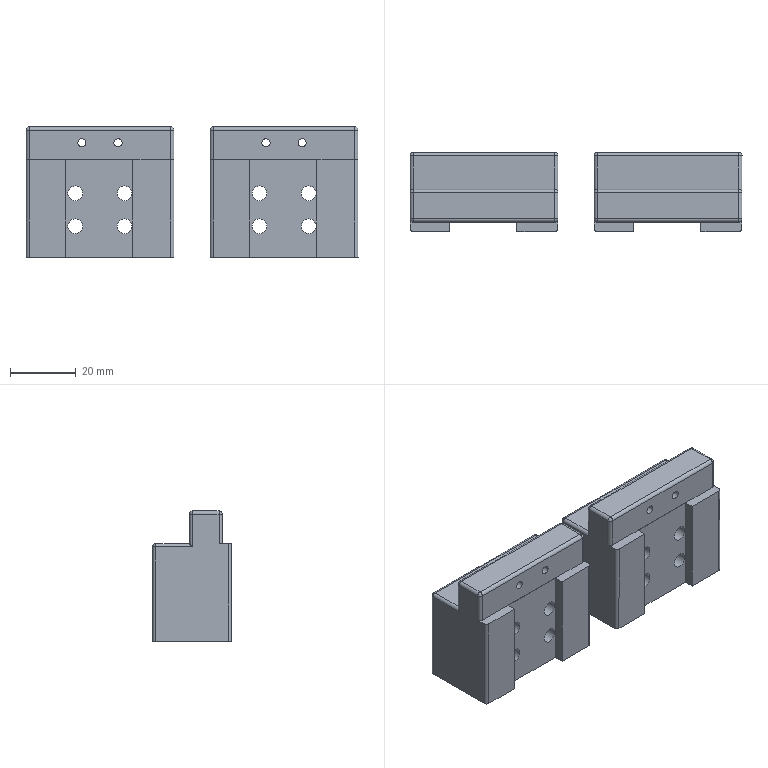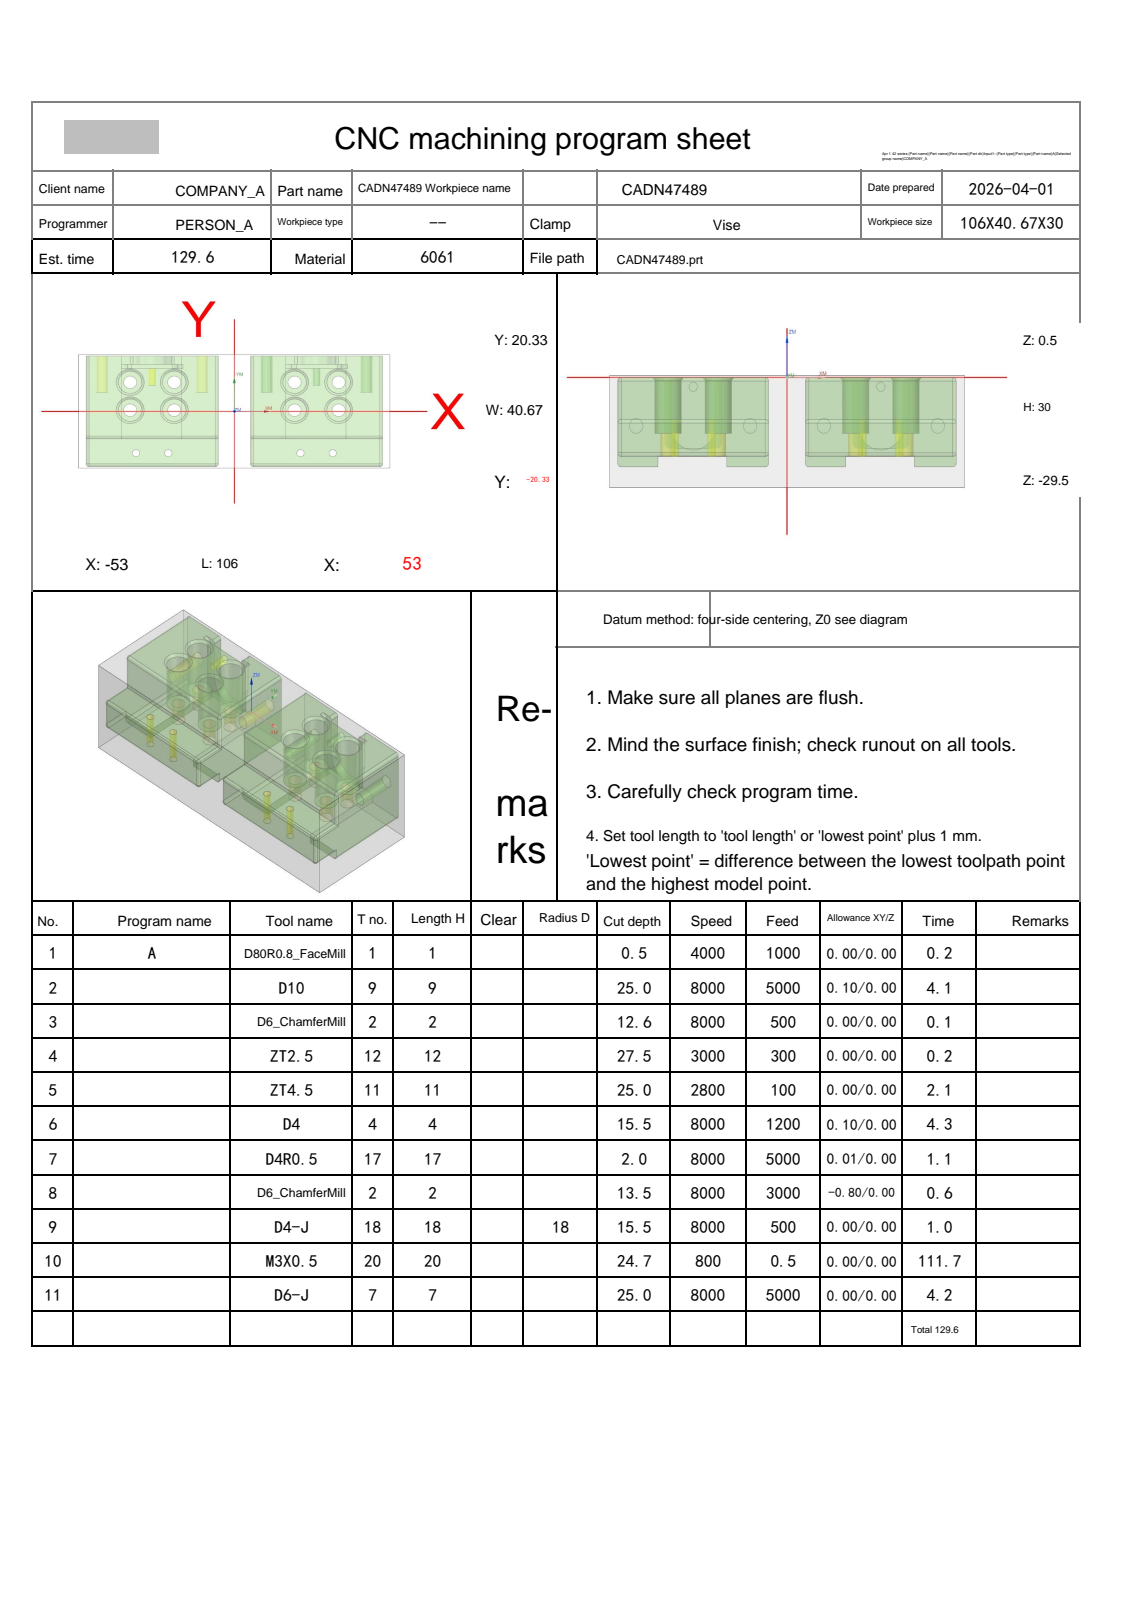NC program | NX | posted by the shop | part box 101.001 x 24.001 x 39.667 mm
Lines 24073 to 26071 of 28944, first 1764 of 1999 lines:
N9 T18 M06
(D4-J  D=4. R=0. H=18 ce=0.00 di=0.00)
G00 G90 G54 X35.5 Y.416 M03 S8000
G43 H18 Z20.
M08
Z.499
G41 D18
G01 X35.54 Y.22 F500.
X35.586 Y.055
X35.662 Y-.098
X35.763 Y-.237
X35.887 Y-.356
X36.029 Y-.451
X36.186 Y-.521
X36.352 Y-.563
X36.523 Y-.576
X36.694 Y-.558
X36.859 Y-.512
X37.014 Y-.438
X37.153 Y-.339
X37.274 Y-.217
X37.371 Y-.076
X37.443 Y.08
X37.487 Y.246
X37.5 Y.416
X37.486 Y.667 Z.399
X37.439 Y.914 Z.299
X37.361 Y1.153 Z.199
X37.254 Y1.381 Z.099
X37.12 Y1.593 Z-.001
X36.959 Y1.787 Z-.101
X36.776 Y1.959 Z-.201
X36.573 Y2.107 Z-.301
X36.352 Y2.228 Z-.401
X36.119 Y2.32 Z-.501
X35.875 Y2.383 Z-.601
X35.626 Y2.414 Z-.701
X35.374 Z-.801
X35.125 Y2.383 Z-.901
X34.881 Y2.32 Z-1.001
X34.648 Y2.228 Z-1.101
X34.427 Y2.107 Z-1.201
X34.224 Y1.959 Z-1.301
X34.041 Y1.787 Z-1.401
X33.88 Y1.593 Z-1.501
X33.746 Y1.381 Z-1.601
X33.639 Y1.153 Z-1.701
X33.561 Y.914 Z-1.801
X33.514 Y.667 Z-1.901
X33.498 Y.416 Z-2.001
X33.514 Y.166 Z-2.101
X33.561 Y-.081 Z-2.201
X33.639 Y-.321 Z-2.301
X33.746 Y-.548 Z-2.401
X33.88 Y-.76 Z-2.501
X34.041 Y-.954 Z-2.601
X34.224 Y-1.126 Z-2.701
X34.427 Y-1.274 Z-2.801
X34.648 Y-1.395 Z-2.901
X34.881 Y-1.488 Z-3.001
X35.125 Y-1.55 Z-3.101
X35.374 Y-1.582 Z-3.201
X35.626 Z-3.301
X35.875 Y-1.55 Z-3.401
X36.119 Y-1.488 Z-3.501
X36.352 Y-1.395 Z-3.601
X36.573 Y-1.274 Z-3.701
X36.776 Y-1.126 Z-3.801
X36.959 Y-.954 Z-3.901
X37.12 Y-.76 Z-4.001
X37.254 Y-.548 Z-4.101
X37.361 Y-.32 Z-4.201
X37.439 Y-.081 Z-4.301
X37.486 Y.166 Z-4.401
X37.502 Y.417 Z-4.501
X37.486 Y.667 Z-4.601
X37.439 Y.914 Z-4.701
X37.361 Y1.154 Z-4.801
X37.254 Y1.381 Z-4.901
X37.12 Y1.593 Z-5.001
X36.959 Y1.787 Z-5.101
X36.776 Y1.959 Z-5.201
X36.573 Y2.107 Z-5.301
X36.352 Y2.228 Z-5.401
X36.119 Y2.321 Z-5.501
X35.875 Y2.383 Z-5.601
X35.626 Y2.415 Z-5.701
X35.374 Z-5.801
X35.125 Y2.383 Z-5.901
X34.881 Y2.321 Z-6.001
X34.648 Y2.228 Z-6.101
X34.427 Y2.107 Z-6.201
X34.224 Y1.959 Z-6.301
X34.041 Y1.787 Z-6.401
X33.88 Y1.593 Z-6.501
X33.746 Y1.381 Z-6.601
X33.639 Y1.154 Z-6.701
X33.561 Y.914 Z-6.801
X33.514 Y.668 Z-6.901
X33.498 Y.417 Z-7.001
X33.514 Y.166 Z-7.101
X33.561 Y-.081 Z-7.201
X33.639 Y-.32 Z-7.301
X33.746 Y-.548 Z-7.401
X33.88 Y-.76 Z-7.501
X34.041 Y-.954 Z-7.601
X34.224 Y-1.126 Z-7.701
X34.427 Y-1.274 Z-7.801
X34.648 Y-1.395 Z-7.901
X34.881 Y-1.487 Z-8.001
X35.125 Y-1.55 Z-8.101
X35.374 Y-1.581 Z-8.201
X35.626 Z-8.301
X35.875 Y-1.55 Z-8.401
X36.119 Y-1.487 Z-8.501
X36.352 Y-1.395 Z-8.601
X36.573 Y-1.274 Z-8.701
X36.776 Y-1.126 Z-8.801
X36.959 Y-.954 Z-8.901
X37.12 Y-.76 Z-9.001
X37.254 Y-.548 Z-9.101
X37.361 Y-.32 Z-9.201
X37.439 Y-.081 Z-9.301
X37.486 Y.166 Z-9.401
X37.502 Y.417 Z-9.501
X37.486 Y.668 Z-9.601
X37.439 Y.915 Z-9.701
X37.361 Y1.154 Z-9.801
X37.254 Y1.381 Z-9.901
X37.12 Y1.593 Z-10.001
X36.959 Y1.787 Z-10.101
X36.776 Y1.959 Z-10.201
X36.573 Y2.107 Z-10.301
X36.352 Y2.228 Z-10.401
X36.119 Y2.321 Z-10.501
X35.875 Y2.383 Z-10.601
X35.626 Y2.415 Z-10.701
X35.374 Z-10.801
X35.125 Y2.383 Z-10.901
X34.881 Y2.321 Z-11.001
X34.648 Y2.228 Z-11.101
X34.427 Y2.107 Z-11.201
X34.224 Y1.959 Z-11.301
X34.041 Y1.787 Z-11.401
X33.88 Y1.594 Z-11.501
X33.746 Y1.381 Z-11.601
X33.639 Y1.154 Z-11.701
X33.561 Y.915 Z-11.801
X33.514 Y.668 Z-11.901
X33.498 Y.417 Z-12.001
X33.514 Y.166 Z-12.101
X33.561 Y-.081 Z-12.201
X33.639 Y-.32 Z-12.301
X33.746 Y-.548 Z-12.401
X33.88 Y-.76 Z-12.501
X34.041 Y-.954 Z-12.601
X34.224 Y-1.126 Z-12.701
X34.427 Y-1.274 Z-12.801
X34.648 Y-1.395 Z-12.901
X34.881 Y-1.487 Z-13.001
X35.125 Y-1.55 Z-13.101
X35.374 Y-1.581 Z-13.201
X35.626 Z-13.301
X35.875 Y-1.55 Z-13.401
X36.119 Y-1.487 Z-13.501
X36.352 Y-1.395 Z-13.601
X36.573 Y-1.273 Z-13.701
X36.776 Y-1.126 Z-13.801
X36.959 Y-.954 Z-13.901
X37.12 Y-.76 Z-14.001
X37.254 Y-.548 Z-14.101
X37.361 Y-.32 Z-14.201
X37.439 Y-.081 Z-14.301
X37.486 Y.166 Z-14.401
X37.502 Y.417 Z-14.501
X37.486 Y.668 Z-14.601
X37.439 Y.915 Z-14.701
X37.361 Y1.154 Z-14.801
X37.254 Y1.381 Z-14.901
X37.118 Y1.592 Z-15.001
X36.959 Y1.787
X36.776 Y1.959
X36.573 Y2.107
X36.352 Y2.228
X36.119 Y2.321
X35.875 Y2.383
X35.626 Y2.415
X35.374
X35.125 Y2.383
X34.881 Y2.321
X34.648 Y2.228
X34.427 Y2.107
X34.224 Y1.959
X34.041 Y1.787
X33.88 Y1.594
X33.746 Y1.381
X33.639 Y1.154
X33.561 Y.915
X33.514 Y.668
X33.498 Y.417
X33.514 Y.166
X33.561 Y-.081
X33.639 Y-.32
X33.746 Y-.548
X33.88 Y-.76
X34.041 Y-.954
X34.224 Y-1.126
X34.427 Y-1.273
X34.648 Y-1.395
X34.881 Y-1.487
X35.125 Y-1.55
X35.374 Y-1.581
X35.626
X35.875 Y-1.55
X36.119 Y-1.487
X36.352 Y-1.395
X36.573 Y-1.273
X36.776 Y-1.126
X36.959 Y-.954
X37.12 Y-.76
X37.254 Y-.548
X37.361 Y-.32
X37.439 Y-.081
X37.486 Y.166
X37.502 Y.417
X37.486 Y.668
X37.439 Y.915
X37.361 Y1.154
X37.254 Y1.381
X37.118 Y1.592
X37.007 Y1.723
X36.874 Y1.831
X36.725 Y1.915
X36.563 Y1.972
X36.394 Y2.
X36.222 Y1.998
X36.053 Y1.967
X35.893 Y1.907
X35.745 Y1.821
X35.614 Y1.71
X35.504 Y1.578
X35.418 Y1.43
X35.359 Y1.269
X35.329 Y1.1
X35.328 Y.928
X35.357 Y.759
X35.417 Y.599
G40 X35.5 Y.417
G00 Z20.
Y.416
Y10.416
Z.499
G41 D18
G01 X35.54 Y10.22
X35.586 Y10.055
X35.662 Y9.902
X35.763 Y9.763
X35.887 Y9.644
X36.029 Y9.549
X36.186 Y9.479
X36.352 Y9.437
X36.523 Y9.424
X36.694 Y9.442
X36.859 Y9.488
X37.014 Y9.562
X37.153 Y9.661
X37.274 Y9.783
X37.371 Y9.924
X37.443 Y10.08
X37.487 Y10.246
X37.5 Y10.416
X37.486 Y10.667 Z.399
X37.439 Y10.914 Z.299
X37.362 Y11.153 Z.199
X37.255 Y11.381 Z.099
X37.12 Y11.593 Z-.001
X36.96 Y11.787 Z-.101
X36.776 Y11.959 Z-.201
X36.573 Y12.107 Z-.301
X36.353 Y12.228 Z-.401
X36.119 Y12.32 Z-.501
X35.875 Y12.383 Z-.601
X35.626 Y12.414 Z-.701
X35.375 Z-.801
X35.125 Y12.383 Z-.901
X34.882 Y12.32 Z-1.001
X34.648 Y12.228 Z-1.101
X34.427 Y12.107 Z-1.201
X34.224 Y11.959 Z-1.301
X34.041 Y11.787 Z-1.401
X33.881 Y11.593 Z-1.501
X33.746 Y11.381 Z-1.601
X33.639 Y11.153 Z-1.701
X33.561 Y10.914 Z-1.801
X33.514 Y10.667 Z-1.901
X33.498 Y10.416 Z-2.001
X33.514 Y10.166 Z-2.101
X33.561 Y9.919 Z-2.201
X33.639 Y9.679 Z-2.301
X33.746 Y9.452 Z-2.401
X33.881 Y9.24 Z-2.501
X34.041 Y9.046 Z-2.601
X34.224 Y8.874 Z-2.701
X34.427 Y8.726 Z-2.801
X34.648 Y8.605 Z-2.901
X34.882 Y8.512 Z-3.001
X35.125 Y8.45 Z-3.101
X35.374 Y8.418 Z-3.201
X35.626 Z-3.301
X35.875 Y8.45 Z-3.401
X36.119 Y8.512 Z-3.501
X36.353 Y8.605 Z-3.601
X36.573 Y8.726 Z-3.701
X36.776 Y8.874 Z-3.801
X36.96 Y9.046 Z-3.901
X37.12 Y9.24 Z-4.001
X37.255 Y9.452 Z-4.101
X37.362 Y9.68 Z-4.201
X37.439 Y9.919 Z-4.301
X37.486 Y10.166 Z-4.401
X37.502 Y10.417 Z-4.501
X37.486 Y10.667 Z-4.601
X37.439 Y10.914 Z-4.701
X37.362 Y11.154 Z-4.801
X37.255 Y11.381 Z-4.901
X37.12 Y11.593 Z-5.001
X36.96 Y11.787 Z-5.101
X36.776 Y11.959 Z-5.201
X36.573 Y12.107 Z-5.301
X36.353 Y12.228 Z-5.401
X36.119 Y12.321 Z-5.501
X35.875 Y12.383 Z-5.601
X35.626 Y12.415 Z-5.701
X35.374 Z-5.801
X35.125 Y12.383 Z-5.901
X34.882 Y12.321 Z-6.001
X34.648 Y12.228 Z-6.101
X34.427 Y12.107 Z-6.201
X34.224 Y11.959 Z-6.301
X34.041 Y11.787 Z-6.401
X33.881 Y11.593 Z-6.501
X33.746 Y11.381 Z-6.601
X33.639 Y11.154 Z-6.701
X33.561 Y10.914 Z-6.801
X33.514 Y10.668 Z-6.901
X33.498 Y10.417 Z-7.001
X33.514 Y10.166 Z-7.101
X33.561 Y9.919 Z-7.201
X33.639 Y9.68 Z-7.301
X33.746 Y9.452 Z-7.401
X33.881 Y9.24 Z-7.501
X34.041 Y9.046 Z-7.601
X34.224 Y8.874 Z-7.701
X34.427 Y8.726 Z-7.801
X34.648 Y8.605 Z-7.901
X34.882 Y8.513 Z-8.001
X35.125 Y8.45 Z-8.101
X35.374 Y8.419 Z-8.201
X35.626 Z-8.301
X35.875 Y8.45 Z-8.401
X36.119 Y8.513 Z-8.501
X36.353 Y8.605 Z-8.601
X36.573 Y8.726 Z-8.701
X36.776 Y8.874 Z-8.801
X36.96 Y9.046 Z-8.901
X37.12 Y9.24 Z-9.001
X37.255 Y9.452 Z-9.101
X37.362 Y9.68 Z-9.201
X37.439 Y9.919 Z-9.301
X37.486 Y10.166 Z-9.401
X37.502 Y10.417 Z-9.501
X37.486 Y10.668 Z-9.601
X37.439 Y10.915 Z-9.701
X37.362 Y11.154 Z-9.801
X37.255 Y11.381 Z-9.901
X37.12 Y11.593 Z-10.001
X36.96 Y11.787 Z-10.101
X36.776 Y11.959 Z-10.201
X36.573 Y12.107 Z-10.301
X36.353 Y12.228 Z-10.401
X36.119 Y12.321 Z-10.501
X35.875 Y12.383 Z-10.601
X35.626 Y12.415 Z-10.701
X35.374 Z-10.801
X35.125 Y12.383 Z-10.901
X34.882 Y12.321 Z-11.001
X34.648 Y12.228 Z-11.101
X34.427 Y12.107 Z-11.201
X34.224 Y11.959 Z-11.301
X34.041 Y11.787 Z-11.401
X33.881 Y11.594 Z-11.501
X33.746 Y11.381 Z-11.601
X33.639 Y11.154 Z-11.701
X33.561 Y10.915 Z-11.801
X33.514 Y10.668 Z-11.901
X33.498 Y10.417 Z-12.001
X33.514 Y10.166 Z-12.101
X33.561 Y9.919 Z-12.201
X33.639 Y9.68 Z-12.301
X33.746 Y9.452 Z-12.401
X33.881 Y9.24 Z-12.501
X34.041 Y9.046 Z-12.601
X34.224 Y8.874 Z-12.701
X34.427 Y8.726 Z-12.801
X34.648 Y8.605 Z-12.901
X34.882 Y8.513 Z-13.001
X35.125 Y8.45 Z-13.101
X35.374 Y8.419 Z-13.201
X35.626 Z-13.301
X35.875 Y8.45 Z-13.401
X36.119 Y8.513 Z-13.501
X36.353 Y8.605 Z-13.601
X36.573 Y8.727 Z-13.701
X36.776 Y8.874 Z-13.801
X36.96 Y9.046 Z-13.901
X37.12 Y9.24 Z-14.001
X37.255 Y9.452 Z-14.101
X37.362 Y9.68 Z-14.201
X37.439 Y9.919 Z-14.301
X37.486 Y10.166 Z-14.401
X37.502 Y10.417 Z-14.501
X37.486 Y10.668 Z-14.601
X37.439 Y10.915 Z-14.701
X37.362 Y11.154 Z-14.801
X37.255 Y11.381 Z-14.901
X37.118 Y11.592 Z-15.001
X36.96 Y11.787
X36.776 Y11.959
X36.573 Y12.107
X36.353 Y12.228
X36.119 Y12.321
X35.875 Y12.383
X35.626 Y12.415
X35.374
X35.125 Y12.383
X34.881 Y12.321
X34.648 Y12.228
X34.427 Y12.107
X34.224 Y11.959
X34.041 Y11.787
X33.88 Y11.594
X33.746 Y11.381
X33.639 Y11.154
X33.561 Y10.915
X33.514 Y10.668
X33.498 Y10.417
X33.514 Y10.166
X33.561 Y9.919
X33.639 Y9.68
X33.746 Y9.452
X33.88 Y9.24
X34.041 Y9.046
X34.224 Y8.874
X34.427 Y8.727
X34.648 Y8.605
X34.881 Y8.513
X35.125 Y8.45
X35.374 Y8.419
X35.626
X35.875 Y8.45
X36.119 Y8.513
X36.353 Y8.605
X36.573 Y8.727
X36.776 Y8.874
X36.96 Y9.046
X37.12 Y9.24
X37.255 Y9.452
X37.362 Y9.68
X37.439 Y9.919
X37.486 Y10.166
X37.502 Y10.417
X37.486 Y10.668
X37.439 Y10.915
X37.362 Y11.154
X37.255 Y11.381
X37.118 Y11.592
X37.007 Y11.723
X36.874 Y11.831
X36.725 Y11.915
X36.563 Y11.972
X36.394 Y12.
X36.222 Y11.998
X36.054 Y11.967
X35.893 Y11.907
X35.745 Y11.821
X35.614 Y11.71
X35.504 Y11.578
X35.418 Y11.43
X35.359 Y11.269
X35.329 Y11.1
Y10.928
X35.358 Y10.759
X35.417 Y10.599
G40 X35.5 Y10.417
G00 Z20.
Y10.416
X20.5
Y10.417
Z.499
G41 D18
G01 X20.54 Y10.221
X20.586 Y10.056
X20.662 Y9.902
X20.763 Y9.764
X20.887 Y9.645
X21.029 Y9.549
X21.186 Y9.479
X21.352 Y9.437
X21.523 Y9.425
X21.694 Y9.442
X21.859 Y9.488
X22.014 Y9.562
X22.153 Y9.661
X22.274 Y9.783
X22.371 Y9.924
X22.443 Y10.08
X22.487 Y10.246
X22.5 Y10.417
X22.486 Y10.668 Z.399
X22.439 Y10.914 Z.299
X22.362 Y11.154 Z.199
X22.255 Y11.381 Z.099
X22.12 Y11.593 Z-.001
X21.96 Y11.787 Z-.101
X21.776 Y11.959 Z-.201
X21.573 Y12.107 Z-.301
X21.353 Y12.228 Z-.401
X21.119 Y12.321 Z-.501
X20.875 Y12.383 Z-.601
X20.626 Y12.415 Z-.701
X20.375 Z-.801
X20.125 Y12.383 Z-.901
X19.882 Y12.321 Z-1.001
X19.648 Y12.228 Z-1.101
X19.427 Y12.107 Z-1.201
X19.224 Y11.959 Z-1.301
X19.041 Y11.787 Z-1.401
X18.881 Y11.593 Z-1.501
X18.746 Y11.381 Z-1.601
X18.639 Y11.154 Z-1.701
X18.561 Y10.915 Z-1.801
X18.514 Y10.668 Z-1.901
X18.498 Y10.417 Z-2.001
X18.514 Y10.166 Z-2.101
X18.561 Y9.919 Z-2.201
X18.639 Y9.68 Z-2.301
X18.746 Y9.452 Z-2.401
X18.881 Y9.24 Z-2.501
X19.041 Y9.046 Z-2.601
X19.224 Y8.874 Z-2.701
X19.427 Y8.726 Z-2.801
X19.648 Y8.605 Z-2.901
X19.882 Y8.513 Z-3.001
X20.125 Y8.45 Z-3.101
X20.374 Y8.419 Z-3.201
X20.626 Z-3.301
X20.875 Y8.45 Z-3.401
X21.119 Y8.513 Z-3.501
X21.353 Y8.605 Z-3.601
X21.573 Y8.726 Z-3.701
X21.776 Y8.874 Z-3.801
X21.96 Y9.046 Z-3.901
X22.12 Y9.24 Z-4.001
X22.255 Y9.452 Z-4.101
X22.362 Y9.68 Z-4.201
X22.439 Y9.919 Z-4.301
X22.486 Y10.166 Z-4.401
X22.502 Y10.417 Z-4.501
X22.486 Y10.668 Z-4.601
X22.439 Y10.915 Z-4.701
X22.362 Y11.154 Z-4.801
X22.255 Y11.381 Z-4.901
X22.12 Y11.594 Z-5.001
X21.96 Y11.787 Z-5.101
X21.776 Y11.959 Z-5.201
X21.573 Y12.107 Z-5.301
X21.353 Y12.228 Z-5.401
X21.119 Y12.321 Z-5.501
X20.875 Y12.383 Z-5.601
X20.626 Y12.415 Z-5.701
X20.374 Z-5.801
X20.125 Y12.383 Z-5.901
X19.882 Y12.321 Z-6.001
X19.648 Y12.228 Z-6.101
X19.427 Y12.107 Z-6.201
X19.224 Y11.959 Z-6.301
X19.041 Y11.787 Z-6.401
X18.881 Y11.594 Z-6.501
X18.746 Y11.381 Z-6.601
X18.639 Y11.154 Z-6.701
X18.561 Y10.915 Z-6.801
X18.514 Y10.668 Z-6.901
X18.498 Y10.417 Z-7.001
X18.514 Y10.166 Z-7.101
X18.561 Y9.919 Z-7.201
X18.639 Y9.68 Z-7.301
X18.746 Y9.452 Z-7.401
X18.881 Y9.24 Z-7.501
X19.041 Y9.046 Z-7.601
X19.224 Y8.874 Z-7.701
X19.427 Y8.727 Z-7.801
X19.648 Y8.605 Z-7.901
X19.882 Y8.513 Z-8.001
X20.125 Y8.45 Z-8.101
X20.374 Y8.419 Z-8.201
X20.626 Z-8.301
X20.875 Y8.45 Z-8.401
X21.119 Y8.513 Z-8.501
X21.353 Y8.605 Z-8.601
X21.573 Y8.727 Z-8.701
X21.776 Y8.874 Z-8.801
X21.96 Y9.046 Z-8.901
X22.12 Y9.24 Z-9.001
X22.255 Y9.452 Z-9.101
X22.362 Y9.68 Z-9.201
X22.439 Y9.919 Z-9.301
X22.486 Y10.166 Z-9.401
X22.502 Y10.417 Z-9.501
X22.486 Y10.668 Z-9.601
X22.439 Y10.915 Z-9.701
X22.362 Y11.154 Z-9.801
X22.255 Y11.381 Z-9.901
X22.12 Y11.594 Z-10.001
X21.96 Y11.787 Z-10.101
X21.776 Y11.96 Z-10.201
X21.573 Y12.107 Z-10.301
X21.353 Y12.228 Z-10.401
X21.119 Y12.321 Z-10.501
X20.875 Y12.384 Z-10.601
X20.626 Y12.415 Z-10.701
X20.374 Z-10.801
X20.125 Y12.384 Z-10.901
X19.882 Y12.321 Z-11.001
X19.648 Y12.228 Z-11.101
X19.427 Y12.107 Z-11.201
X19.224 Y11.96 Z-11.301
X19.041 Y11.787 Z-11.401
X18.881 Y11.594 Z-11.501
X18.746 Y11.381 Z-11.601
X18.639 Y11.154 Z-11.701
X18.561 Y10.915 Z-11.801
X18.514 Y10.668 Z-11.901
X18.498 Y10.417 Z-12.001
X18.514 Y10.166 Z-12.101
X18.561 Y9.919 Z-12.201
X18.639 Y9.68 Z-12.301
X18.746 Y9.453 Z-12.401
X18.881 Y9.24 Z-12.501
X19.041 Y9.047 Z-12.601
X19.224 Y8.874 Z-12.701
X19.427 Y8.727 Z-12.801
X19.648 Y8.606 Z-12.901
X19.882 Y8.513 Z-13.001
X20.125 Y8.451 Z-13.101
X20.374 Y8.419 Z-13.201
X20.626 Z-13.301
X20.875 Y8.451 Z-13.401
X21.119 Y8.513 Z-13.501
X21.353 Y8.606 Z-13.601
X21.573 Y8.727 Z-13.701
X21.776 Y8.875 Z-13.801
X21.96 Y9.047 Z-13.901
X22.12 Y9.24 Z-14.001
X22.255 Y9.453 Z-14.101
X22.362 Y9.68 Z-14.201
X22.439 Y9.919 Z-14.301
X22.486 Y10.166 Z-14.401
X22.502 Y10.417 Z-14.501
X22.486 Y10.668 Z-14.601
X22.439 Y10.915 Z-14.701
X22.362 Y11.154 Z-14.801
X22.255 Y11.382 Z-14.901
X22.118 Y11.593 Z-15.001
X21.96 Y11.788
X21.776 Y11.96
X21.573 Y12.107
X21.353 Y12.229
X21.119 Y12.321
X20.875 Y12.384
X20.626 Y12.415
X20.374
X20.125 Y12.384
X19.881 Y12.321
X19.648 Y12.229
X19.427 Y12.107
X19.224 Y11.96
X19.041 Y11.788
X18.88 Y11.594
X18.746 Y11.382
X18.639 Y11.154
X18.561 Y10.915
X18.514 Y10.668
X18.498 Y10.417
X18.514 Y10.166
X18.561 Y9.919
X18.639 Y9.68
X18.746 Y9.453
X18.88 Y9.24
X19.041 Y9.047
X19.224 Y8.875
X19.427 Y8.727
X19.648 Y8.606
X19.881 Y8.513
X20.125 Y8.451
X20.374 Y8.419
X20.626
X20.875 Y8.451
X21.119 Y8.513
X21.353 Y8.606
X21.573 Y8.727
X21.776 Y8.875
X21.96 Y9.047
X22.12 Y9.24
X22.255 Y9.453
X22.362 Y9.68
X22.439 Y9.919
X22.486 Y10.166
X22.502 Y10.417
X22.486 Y10.668
X22.439 Y10.915
X22.362 Y11.154
X22.255 Y11.382
X22.118 Y11.593
X22.007 Y11.723
X21.874 Y11.832
X21.725 Y11.915
X21.563 Y11.972
X21.394 Y12.
X21.222 Y11.998
X21.054 Y11.967
X20.893 Y11.907
X20.745 Y11.821
X20.614 Y11.71
X20.504 Y11.579
X20.418 Y11.43
X20.359 Y11.269
X20.329 Y11.1
Y10.929
X20.358 Y10.76
X20.417 Y10.599
G40 X20.5 Y10.417
G00 Z20.
Y10.416
Y.416
Y.417
Z.499
G41 D18
G01 X20.54 Y.221
X20.586 Y.056
X20.662 Y-.098
X20.763 Y-.236
X20.887 Y-.355
X21.029 Y-.451
X21.186 Y-.521
X21.352 Y-.563
X21.523 Y-.575
X21.694 Y-.558
X21.859 Y-.512
X22.014 Y-.438
X22.153 Y-.339
X22.274 Y-.217
X22.371 Y-.076
X22.443 Y.08
X22.487 Y.246
X22.5 Y.417
X22.486 Y.668 Z.399
X22.439 Y.914 Z.299
X22.361 Y1.154 Z.199
X22.254 Y1.381 Z.099
X22.12 Y1.593 Z-.001
X21.959 Y1.787 Z-.101
X21.776 Y1.959 Z-.201
X21.573 Y2.107 Z-.301
X21.352 Y2.228 Z-.401
X21.119 Y2.321 Z-.501
X20.875 Y2.383 Z-.601
X20.626 Y2.415 Z-.701
X20.374 Z-.801
X20.125 Y2.383 Z-.901
X19.881 Y2.321 Z-1.001
X19.648 Y2.228 Z-1.101
X19.427 Y2.107 Z-1.201
X19.224 Y1.959 Z-1.301
X19.041 Y1.787 Z-1.401
X18.88 Y1.593 Z-1.501
X18.746 Y1.381 Z-1.601
X18.639 Y1.154 Z-1.701
X18.561 Y.915 Z-1.801
X18.514 Y.668 Z-1.901
X18.498 Y.417 Z-2.001
X18.514 Y.166 Z-2.101
X18.561 Y-.081 Z-2.201
X18.639 Y-.32 Z-2.301
X18.746 Y-.548 Z-2.401
X18.88 Y-.76 Z-2.501
X19.041 Y-.954 Z-2.601
X19.224 Y-1.126 Z-2.701
X19.427 Y-1.274 Z-2.801
X19.648 Y-1.395 Z-2.901
X19.881 Y-1.487 Z-3.001
X20.125 Y-1.55 Z-3.101
X20.374 Y-1.581 Z-3.201
X20.626 Z-3.301
X20.875 Y-1.55 Z-3.401
X21.119 Y-1.487 Z-3.501
X21.352 Y-1.395 Z-3.601
X21.573 Y-1.274 Z-3.701
X21.776 Y-1.126 Z-3.801
X21.959 Y-.954 Z-3.901
X22.12 Y-.76 Z-4.001
X22.254 Y-.548 Z-4.101
X22.361 Y-.32 Z-4.201
X22.439 Y-.081 Z-4.301
X22.486 Y.166 Z-4.401
X22.502 Y.417 Z-4.501
X22.486 Y.668 Z-4.601
X22.439 Y.915 Z-4.701
X22.361 Y1.154 Z-4.801
X22.254 Y1.381 Z-4.901
X22.12 Y1.594 Z-5.001
X21.959 Y1.787 Z-5.101
X21.776 Y1.959 Z-5.201
X21.573 Y2.107 Z-5.301
X21.352 Y2.228 Z-5.401
X21.119 Y2.321 Z-5.501
X20.875 Y2.383 Z-5.601
X20.626 Y2.415 Z-5.701
X20.374 Z-5.801
X20.125 Y2.383 Z-5.901
X19.881 Y2.321 Z-6.001
X19.648 Y2.228 Z-6.101
X19.427 Y2.107 Z-6.201
X19.224 Y1.959 Z-6.301
X19.041 Y1.787 Z-6.401
X18.88 Y1.594 Z-6.501
X18.746 Y1.381 Z-6.601
X18.639 Y1.154 Z-6.701
X18.561 Y.915 Z-6.801
X18.514 Y.668 Z-6.901
X18.498 Y.417 Z-7.001
X18.514 Y.166 Z-7.101
X18.561 Y-.081 Z-7.201
X18.639 Y-.32 Z-7.301
X18.746 Y-.548 Z-7.401
X18.88 Y-.76 Z-7.501
X19.041 Y-.954 Z-7.601
X19.224 Y-1.126 Z-7.701
X19.427 Y-1.273 Z-7.801
X19.648 Y-1.395 Z-7.901
X19.881 Y-1.487 Z-8.001
X20.125 Y-1.55 Z-8.101
X20.374 Y-1.581 Z-8.201
X20.626 Z-8.301
X20.875 Y-1.55 Z-8.401
X21.119 Y-1.487 Z-8.501
X21.352 Y-1.395 Z-8.601
X21.573 Y-1.273 Z-8.701
X21.776 Y-1.126 Z-8.801
X21.959 Y-.954 Z-8.901
X22.12 Y-.76 Z-9.001
X22.254 Y-.548 Z-9.101
X22.361 Y-.32 Z-9.201
X22.439 Y-.081 Z-9.301
X22.486 Y.166 Z-9.401
X22.502 Y.417 Z-9.501
X22.486 Y.668 Z-9.601
X22.439 Y.915 Z-9.701
X22.361 Y1.154 Z-9.801
X22.254 Y1.381 Z-9.901
X22.12 Y1.594 Z-10.001
X21.959 Y1.787 Z-10.101
X21.776 Y1.96 Z-10.201
X21.573 Y2.107 Z-10.301
X21.352 Y2.228 Z-10.401
X21.119 Y2.321 Z-10.501
X20.875 Y2.384 Z-10.601
X20.626 Y2.415 Z-10.701
X20.374 Z-10.801
X20.125 Y2.384 Z-10.901
X19.881 Y2.321 Z-11.001
X19.648 Y2.228 Z-11.101
X19.427 Y2.107 Z-11.201
X19.224 Y1.96 Z-11.301
X19.041 Y1.787 Z-11.401
X18.88 Y1.594 Z-11.501
X18.746 Y1.381 Z-11.601
X18.639 Y1.154 Z-11.701
X18.561 Y.915 Z-11.801
X18.514 Y.668 Z-11.901
X18.498 Y.417 Z-12.001
X18.514 Y.166 Z-12.101
X18.561 Y-.081 Z-12.201
X18.639 Y-.32 Z-12.301
X18.746 Y-.547 Z-12.401
X18.88 Y-.76 Z-12.501
X19.041 Y-.953 Z-12.601
X19.224 Y-1.126 Z-12.701
X19.427 Y-1.273 Z-12.801
X19.648 Y-1.394 Z-12.901
X19.881 Y-1.487 Z-13.001
X20.125 Y-1.549 Z-13.101
X20.374 Y-1.581 Z-13.201
X20.626 Z-13.301
X20.875 Y-1.549 Z-13.401
X21.119 Y-1.487 Z-13.501
X21.352 Y-1.394 Z-13.601
X21.573 Y-1.273 Z-13.701
X21.776 Y-1.125 Z-13.801
X21.959 Y-.953 Z-13.901
X22.12 Y-.76 Z-14.001
X22.254 Y-.547 Z-14.101
X22.361 Y-.32 Z-14.201
X22.439 Y-.081 Z-14.301
X22.486 Y.166 Z-14.401
X22.502 Y.417 Z-14.501
X22.486 Y.668 Z-14.601
X22.439 Y.915 Z-14.701
X22.361 Y1.154 Z-14.801
X22.254 Y1.382 Z-14.901
X22.118 Y1.593 Z-15.001
X21.959 Y1.788
X21.776 Y1.96
X21.573 Y2.107
X21.352 Y2.229
X21.119 Y2.321
X20.875 Y2.384
X20.626 Y2.415
X20.374
X20.125 Y2.384
X19.881 Y2.321
X19.648 Y2.229
X19.427 Y2.107
X19.224 Y1.96
X19.041 Y1.788
X18.88 Y1.594
X18.746 Y1.382
X18.639 Y1.154
X18.561 Y.915
X18.514 Y.668
X18.498 Y.417
X18.514 Y.166
X18.561 Y-.081
X18.639 Y-.32
X18.746 Y-.547
X18.88 Y-.76
X19.041 Y-.953
X19.224 Y-1.125
X19.427 Y-1.273
X19.648 Y-1.394
X19.881 Y-1.487
X20.125 Y-1.549
X20.374 Y-1.581
X20.626
X20.875 Y-1.549
X21.119 Y-1.487
X21.352 Y-1.394
X21.573 Y-1.273
X21.776 Y-1.125
X21.959 Y-.953
X22.12 Y-.76
X22.254 Y-.547
X22.361 Y-.32
X22.439 Y-.081
X22.486 Y.166
X22.502 Y.417
X22.486 Y.668
X22.439 Y.915
X22.361 Y1.154
X22.254 Y1.382
X22.118 Y1.593
X22.007 Y1.723
X21.874 Y1.832
X21.725 Y1.915
X21.563 Y1.972
X21.394 Y2.
X21.222 Y1.998
X21.053 Y1.967
X20.893 Y1.907
X20.745 Y1.821
X20.614 Y1.71
X20.504 Y1.579
X20.418 Y1.43
X20.359 Y1.269
X20.329 Y1.1
X20.328 Y.929
X20.357 Y.76
X20.417 Y.599
G40 X20.5 Y.417
G00 Z20.
Y.416
X-20.5 Y.417
Z.499
G41 D18
G01 X-20.46 Y.221
X-20.414 Y.056
X-20.338 Y-.097
X-20.237 Y-.236
X-20.113 Y-.355
X-19.971 Y-.45
X-19.814 Y-.52
X-19.648 Y-.562
X-19.477 Y-.575
X-19.306 Y-.558
X-19.141 Y-.511
X-18.986 Y-.437
X-18.847 Y-.338
X-18.726 Y-.216
X-18.629 Y-.075
X-18.557 Y.081
X-18.513 Y.246
X-18.5 Y.417
X-18.514 Y.668 Z.399
X-18.561 Y.915 Z.299
X-18.639 Y1.154 Z.199
X-18.746 Y1.382 Z.099
X-18.88 Y1.594 Z-.001
X-19.041 Y1.788 Z-.101
X-19.224 Y1.96 Z-.201
X-19.427 Y2.108 Z-.301
X-19.648 Y2.229 Z-.401
X-19.881 Y2.321 Z-.501
X-20.125 Y2.384 Z-.601
X-20.374 Y2.415 Z-.701
X-20.626 Z-.801
X-20.875 Y2.384 Z-.901
X-21.119 Y2.321 Z-1.001
X-21.352 Y2.229 Z-1.101
X-21.573 Y2.108 Z-1.201
X-21.776 Y1.96 Z-1.301
X-21.959 Y1.788 Z-1.401
X-22.12 Y1.594 Z-1.501
X-22.254 Y1.382 Z-1.601
X-22.361 Y1.154 Z-1.701
X-22.439 Y.915 Z-1.801
X-22.486 Y.668 Z-1.901
X-22.502 Y.417 Z-2.001
X-22.486 Y.166 Z-2.101
X-22.439 Y-.081 Z-2.201
X-22.361 Y-.32 Z-2.301
X-22.254 Y-.547 Z-2.401
X-22.12 Y-.759 Z-2.501
X-21.959 Y-.953 Z-2.601
X-21.776 Y-1.125 Z-2.701
X-21.573 Y-1.273 Z-2.801
X-21.352 Y-1.394 Z-2.901
X-21.119 Y-1.487 Z-3.001
X-20.875 Y-1.549 Z-3.101
X-20.626 Y-1.581 Z-3.201
X-20.374 Z-3.301
X-20.125 Y-1.549 Z-3.401
X-19.881 Y-1.487 Z-3.501
X-19.648 Y-1.394 Z-3.601
X-19.427 Y-1.273 Z-3.701
X-19.224 Y-1.125 Z-3.801
X-19.041 Y-.953 Z-3.901
X-18.88 Y-.759 Z-4.001
X-18.746 Y-.547 Z-4.101
X-18.639 Y-.32 Z-4.201
X-18.561 Y-.08 Z-4.301
X-18.514 Y.167 Z-4.401
X-18.498 Y.417 Z-4.501
X-18.514 Y.668 Z-4.601
X-18.561 Y.915 Z-4.701
X-18.639 Y1.154 Z-4.801
X-18.746 Y1.382 Z-4.901
X-18.88 Y1.594 Z-5.001
X-19.041 Y1.788 Z-5.101
X-19.224 Y1.96 Z-5.201
X-19.427 Y2.108 Z-5.301
X-19.648 Y2.229 Z-5.401
X-19.881 Y2.321 Z-5.501
X-20.125 Y2.384 Z-5.601
X-20.374 Y2.416 Z-5.701
X-20.626 Z-5.801
X-20.875 Y2.384 Z-5.901
X-21.119 Y2.322 Z-6.001
X-21.352 Y2.229 Z-6.101
X-21.573 Y2.108 Z-6.201
X-21.776 Y1.96 Z-6.301
X-21.959 Y1.788 Z-6.401
X-22.12 Y1.594 Z-6.501
X-22.254 Y1.382 Z-6.601
X-22.361 Y1.155 Z-6.701
X-22.439 Y.915 Z-6.801
X-22.486 Y.668 Z-6.901
X-22.502 Y.418 Z-7.001
X-22.486 Y.167 Z-7.101
X-22.439 Y-.08 Z-7.201
X-22.361 Y-.319 Z-7.301
X-22.254 Y-.547 Z-7.401
X-22.12 Y-.759 Z-7.501
X-21.959 Y-.953 Z-7.601
X-21.776 Y-1.125 Z-7.701
X-21.573 Y-1.273 Z-7.801
X-21.352 Y-1.394 Z-7.901
X-21.119 Y-1.486 Z-8.001
X-20.875 Y-1.549 Z-8.101
X-20.626 Y-1.58 Z-8.201
X-20.374 Z-8.301
X-20.125 Y-1.549 Z-8.401
X-19.881 Y-1.486 Z-8.501
X-19.648 Y-1.394 Z-8.601
X-19.427 Y-1.273 Z-8.701
X-19.224 Y-1.125 Z-8.801
X-19.041 Y-.953 Z-8.901
X-18.88 Y-.759 Z-9.001
X-18.746 Y-.547 Z-9.101
X-18.639 Y-.319 Z-9.201
X-18.561 Y-.08 Z-9.301
X-18.514 Y.167 Z-9.401
X-18.498 Y.418 Z-9.501
X-18.514 Y.669 Z-9.601
X-18.561 Y.916 Z-9.701
X-18.639 Y1.155 Z-9.801
X-18.746 Y1.382 Z-9.901
X-18.88 Y1.594 Z-10.001
X-19.041 Y1.788 Z-10.101
X-19.224 Y1.96 Z-10.201
X-19.427 Y2.108 Z-10.301
X-19.648 Y2.229 Z-10.401
X-19.881 Y2.322 Z-10.501
X-20.125 Y2.384 Z-10.601
X-20.374 Y2.416 Z-10.701
X-20.626 Z-10.801
X-20.875 Y2.384 Z-10.901
X-21.119 Y2.322 Z-11.001
X-21.352 Y2.229 Z-11.101
X-21.573 Y2.108 Z-11.201
X-21.776 Y1.96 Z-11.301
X-21.959 Y1.788 Z-11.401
X-22.12 Y1.594 Z-11.501
X-22.254 Y1.382 Z-11.601
X-22.361 Y1.155 Z-11.701
X-22.439 Y.916 Z-11.801
X-22.486 Y.669 Z-11.901
X-22.502 Y.418 Z-12.001
X-22.486 Y.167 Z-12.101
X-22.439 Y-.08 Z-12.201
X-22.361 Y-.319 Z-12.301
X-22.254 Y-.547 Z-12.401
X-22.12 Y-.759 Z-12.501
X-21.959 Y-.953 Z-12.601
X-21.776 Y-1.125 Z-12.701
X-21.573 Y-1.273 Z-12.801
X-21.352 Y-1.394 Z-12.901
X-21.119 Y-1.486 Z-13.001
X-20.875 Y-1.549 Z-13.101
X-20.626 Y-1.58 Z-13.201
X-20.374 Z-13.301
X-20.125 Y-1.549 Z-13.401
X-19.881 Y-1.486 Z-13.501
X-19.648 Y-1.394 Z-13.601
X-19.427 Y-1.273 Z-13.701
X-19.224 Y-1.125 Z-13.801
X-19.041 Y-.953 Z-13.901
X-18.88 Y-.759 Z-14.001
X-18.746 Y-.547 Z-14.101
X-18.639 Y-.319 Z-14.201
X-18.561 Y-.08 Z-14.301
X-18.514 Y.167 Z-14.401
X-18.498 Y.418 Z-14.501
X-18.514 Y.669 Z-14.601
X-18.561 Y.916 Z-14.701
X-18.639 Y1.155 Z-14.801
X-18.746 Y1.382 Z-14.901
X-18.882 Y1.593 Z-15.001
X-19.041 Y1.788
X-19.224 Y1.96
X-19.427 Y2.108
X-19.648 Y2.229
X-19.881 Y2.322
X-20.125 Y2.384
X-20.374 Y2.416
X-20.626
X-20.875 Y2.384
X-21.119 Y2.322
X-21.352 Y2.229
X-21.573 Y2.108
X-21.776 Y1.96
X-21.959 Y1.788
X-22.12 Y1.595
X-22.254 Y1.382
X-22.361 Y1.155
X-22.439 Y.916
X-22.486 Y.669
X-22.502 Y.418
X-22.486 Y.167
X-22.439 Y-.08
X-22.361 Y-.319
X-22.254 Y-.547
X-22.12 Y-.759
X-21.959 Y-.953
X-21.776 Y-1.125
X-21.573 Y-1.273
X-21.352 Y-1.394
X-21.119 Y-1.486
X-20.875 Y-1.549
X-20.626 Y-1.58
X-20.374
X-20.125 Y-1.549
X-19.881 Y-1.486
X-19.648 Y-1.394
X-19.427 Y-1.273
X-19.224 Y-1.125
X-19.041 Y-.953
X-18.88 Y-.759
X-18.746 Y-.547
X-18.639 Y-.319
X-18.561 Y-.08
X-18.514 Y.167
X-18.498 Y.418
X-18.514 Y.669
X-18.561 Y.916
X-18.639 Y1.155
X-18.746 Y1.382
X-18.882 Y1.593
X-18.993 Y1.724
X-19.126 Y1.832
X-19.275 Y1.916
X-19.437 Y1.973
X-19.606 Y2.001
X-19.778 Y1.999
X-19.947 Y1.968
X-20.107 Y1.908
X-20.255 Y1.822
X-20.386 Y1.711
X-20.496 Y1.579
X-20.582 Y1.431
X-20.641 Y1.27
X-20.671 Y1.101
X-20.672 Y.929
X-20.643 Y.76
X-20.583 Y.6
G40 X-20.5 Y.418
G00 Z20.
Y.417
Y10.417
Z.5
G41 D18
G01 X-20.46 Y10.221
X-20.414 Y10.056
X-20.338 Y9.903
X-20.237 Y9.764
X-20.113 Y9.645
X-19.971 Y9.55
X-19.814 Y9.48
X-19.648 Y9.438
X-19.477 Y9.425
X-19.306 Y9.442
X-19.141 Y9.489
X-18.986 Y9.563
X-18.847 Y9.662
X-18.726 Y9.784
X-18.629 Y9.925
X-18.557 Y10.081
X-18.513 Y10.246
X-18.5 Y10.417
X-18.514 Y10.668 Z.4
X-18.561 Y10.915 Z.3
X-18.638 Y11.154 Z.2
X-18.745 Y11.382 Z.1
X-18.88 Y11.594 Z0.0
X-19.04 Y11.788 Z-.1
X-19.224 Y11.96 Z-.2
X-19.427 Y12.108 Z-.3
X-19.647 Y12.229 Z-.4
X-19.881 Y12.321 Z-.5
X-20.125 Y12.384 Z-.6
X-20.374 Y12.415 Z-.7
X-20.625 Z-.8
X-20.875 Y12.384 Z-.9
X-21.118 Y12.321 Z-1.
X-21.352 Y12.229 Z-1.1
X-21.573 Y12.108 Z-1.2
X-21.776 Y11.96 Z-1.3
X-21.959 Y11.788 Z-1.4
X-22.119 Y11.594 Z-1.5
X-22.254 Y11.382 Z-1.6
X-22.361 Y11.154 Z-1.7
X-22.439 Y10.915 Z-1.8
X-22.486 Y10.668 Z-1.9
X-22.502 Y10.417 Z-2.
X-22.486 Y10.166 Z-2.1
X-22.439 Y9.919 Z-2.2
X-22.361 Y9.68 Z-2.3
X-22.254 Y9.453 Z-2.4
X-22.119 Y9.241 Z-2.5
X-21.959 Y9.047 Z-2.6
X-21.776 Y8.875 Z-2.7
X-21.573 Y8.727 Z-2.8
X-21.352 Y8.606 Z-2.901
X-21.118 Y8.513 Z-3.001
X-20.875 Y8.451 Z-3.101
X-20.626 Y8.419 Z-3.201
X-20.374 Z-3.301
X-20.125 Y8.451 Z-3.401
X-19.881 Y8.513 Z-3.501
X-19.647 Y8.606 Z-3.601
X-19.427 Y8.727 Z-3.701
X-19.224 Y8.875 Z-3.801
X-19.04 Y9.047 Z-3.9
X-18.88 Y9.241 Z-4.
X-18.745 Y9.453 Z-4.1
X-18.638 Y9.68 Z-4.2
X-18.561 Y9.92 Z-4.3
X-18.514 Y10.167 Z-4.4
X-18.498 Y10.417 Z-4.5
X-18.514 Y10.668 Z-4.6
X-18.561 Y10.915 Z-4.7
X-18.638 Y11.154 Z-4.8
X-18.745 Y11.382 Z-4.9
X-18.88 Y11.594 Z-5.
X-19.04 Y11.788 Z-5.1
X-19.224 Y11.96 Z-5.2
X-19.427 Y12.108 Z-5.3
X-19.647 Y12.229 Z-5.4
X-19.881 Y12.321 Z-5.5
X-20.125 Y12.384 Z-5.6
X-20.374 Y12.416 Z-5.7
X-20.626 Z-5.8
X-20.875 Y12.384 Z-5.9
X-21.118 Y12.322 Z-6.
X-21.352 Y12.229 Z-6.1
X-21.573 Y12.108 Z-6.2
X-21.776 Y11.96 Z-6.3
X-21.959 Y11.788 Z-6.4
X-22.119 Y11.594 Z-6.5
X-22.254 Y11.382 Z-6.6
X-22.361 Y11.155 Z-6.7
X-22.439 Y10.915 Z-6.8
X-22.486 Y10.668 Z-6.9
X-22.502 Y10.418 Z-7.
X-22.486 Y10.167 Z-7.1
X-22.439 Y9.92 Z-7.2
X-22.361 Y9.681 Z-7.3
X-22.254 Y9.453 Z-7.4
X-22.119 Y9.241 Z-7.5
X-21.959 Y9.047 Z-7.6
X-21.776 Y8.875 Z-7.7
X-21.573 Y8.727 Z-7.8
X-21.352 Y8.606 Z-7.901
X-21.118 Y8.514 Z-8.001
X-20.875 Y8.451 Z-8.101
X-20.626 Y8.42 Z-8.201
X-20.374 Z-8.301
X-20.125 Y8.451 Z-8.401
X-19.881 Y8.514 Z-8.501
X-19.647 Y8.606 Z-8.601
X-19.427 Y8.727 Z-8.701
X-19.224 Y8.875 Z-8.801
X-19.04 Y9.047 Z-8.9
X-18.88 Y9.241 Z-9.
X-18.745 Y9.453 Z-9.1
X-18.638 Y9.681 Z-9.2
X-18.561 Y9.92 Z-9.3
X-18.514 Y10.167 Z-9.4
X-18.498 Y10.418 Z-9.5
X-18.514 Y10.669 Z-9.6
X-18.561 Y10.916 Z-9.7
X-18.638 Y11.155 Z-9.8
X-18.745 Y11.382 Z-9.9
X-18.88 Y11.594 Z-10.
X-19.04 Y11.788 Z-10.1
X-19.224 Y11.96 Z-10.2
X-19.427 Y12.108 Z-10.3
X-19.647 Y12.229 Z-10.4
X-19.881 Y12.322 Z-10.5
X-20.125 Y12.384 Z-10.6
X-20.374 Y12.416 Z-10.7
X-20.626 Z-10.8
X-20.875 Y12.384 Z-10.9
X-21.118 Y12.322 Z-11.
X-21.352 Y12.229 Z-11.1
X-21.573 Y12.108 Z-11.2
X-21.776 Y11.96 Z-11.3
X-21.959 Y11.788 Z-11.4
X-22.119 Y11.594 Z-11.5
X-22.254 Y11.382 Z-11.6
X-22.361 Y11.155 Z-11.7
X-22.439 Y10.916 Z-11.8
X-22.486 Y10.669 Z-11.9
X-22.502 Y10.418 Z-12.
X-22.486 Y10.167 Z-12.1
X-22.439 Y9.92 Z-12.2
X-22.361 Y9.681 Z-12.3
X-22.254 Y9.453 Z-12.4
X-22.119 Y9.241 Z-12.5
X-21.959 Y9.047 Z-12.6
X-21.776 Y8.875 Z-12.7
X-21.573 Y8.727 Z-12.8
X-21.352 Y8.606 Z-12.901
X-21.118 Y8.514 Z-13.001
X-20.875 Y8.451 Z-13.101
X-20.626 Y8.42 Z-13.201
X-20.374 Z-13.301
X-20.125 Y8.451 Z-13.401
X-19.881 Y8.514 Z-13.501
X-19.647 Y8.606 Z-13.601
X-19.427 Y8.727 Z-13.701
X-19.224 Y8.875 Z-13.801
X-19.04 Y9.047 Z-13.9
X-18.88 Y9.241 Z-14.
X-18.745 Y9.453 Z-14.1
X-18.638 Y9.681 Z-14.2
X-18.561 Y9.92 Z-14.3
X-18.514 Y10.167 Z-14.4
X-18.498 Y10.418 Z-14.5
X-18.514 Y10.669 Z-14.6
X-18.561 Y10.916 Z-14.7
X-18.638 Y11.155 Z-14.8
X-18.745 Y11.382 Z-14.9
X-18.882 Y11.593 Z-15.
X-19.04 Y11.788
X-19.224 Y11.96
X-19.427 Y12.108
X-19.647 Y12.229
X-19.881 Y12.322
X-20.125 Y12.384
X-20.374 Y12.416
X-20.626
X-20.875 Y12.384
X-21.119 Y12.322
X-21.352 Y12.229
X-21.573 Y12.108
X-21.776 Y11.96
X-21.959 Y11.788
X-22.12 Y11.595
X-22.254 Y11.382
X-22.361 Y11.155
X-22.439 Y10.916
X-22.486 Y10.669
X-22.502 Y10.418
X-22.486 Y10.167
X-22.439 Y9.92
X-22.361 Y9.681
X-22.254 Y9.453
X-22.12 Y9.241
X-21.959 Y9.047
X-21.776 Y8.875
X-21.573 Y8.727
X-21.352 Y8.606 Z-15.001
X-21.119 Y8.514
X-20.875 Y8.451
X-20.626 Y8.42
X-20.374
X-20.125 Y8.451
X-19.881 Y8.514
X-19.647 Y8.606
X-19.427 Y8.727
X-19.224 Y8.875
X-19.04 Y9.047 Z-15.
X-18.88 Y9.241
X-18.745 Y9.453
X-18.638 Y9.681
X-18.561 Y9.92
X-18.514 Y10.167
X-18.498 Y10.418
X-18.514 Y10.669
X-18.561 Y10.916
X-18.638 Y11.155
X-18.745 Y11.382
X-18.882 Y11.593
X-18.993 Y11.724
X-19.126 Y11.832
X-19.275 Y11.916
X-19.437 Y11.973
X-19.606 Y12.001
X-19.778 Y11.999
X-19.946 Y11.968
X-20.107 Y11.908
X-20.255 Y11.822
X-20.386 Y11.711
X-20.496 Y11.579
X-20.582 Y11.431
X-20.641 Y11.27
X-20.671 Y11.101
Y10.929
X-20.642 Y10.76
X-20.583 Y10.6
G40 X-20.5 Y10.418
G00 Z20.
Y10.417
X-35.5
Y10.418
Z.5
G41 D18
G01 X-35.46 Y10.221
X-35.414 Y10.057
X-35.338 Y9.903
X-35.237 Y9.764
X-35.113 Y9.646
X-34.971 Y9.55
X-34.814 Y9.48
X-34.648 Y9.438
X-34.477 Y9.426
X-34.306 Y9.443
X-34.141 Y9.489
X-33.986 Y9.563
X-33.847 Y9.662
X-33.726 Y9.784
X-33.629 Y9.925
X-33.557 Y10.081
X-33.513 Y10.247
X-33.5 Y10.418
X-33.514 Y10.668 Z.4
X-33.561 Y10.915 Z.3
X-33.638 Y11.155 Z.2
X-33.745 Y11.382 Z.1
X-33.88 Y11.594 Z0.0
X-34.04 Y11.788 Z-.1
X-34.224 Y11.96 Z-.2
X-34.427 Y12.108 Z-.3
X-34.647 Y12.229 Z-.4
X-34.881 Y12.322 Z-.5
X-35.125 Y12.384 Z-.6
X-35.374 Y12.416 Z-.7
X-35.625 Z-.8
X-35.875 Y12.384 Z-.9
X-36.118 Y12.322 Z-1.
X-36.352 Y12.229 Z-1.1
X-36.573 Y12.108 Z-1.2
X-36.776 Y11.96 Z-1.3
X-36.959 Y11.788 Z-1.4
X-37.119 Y11.594 Z-1.5
X-37.254 Y11.382 Z-1.6
X-37.361 Y11.155 Z-1.7
X-37.439 Y10.915 Z-1.8
X-37.486 Y10.669 Z-1.9
X-37.502 Y10.418 Z-2.
X-37.486 Y10.167 Z-2.1
X-37.439 Y9.92 Z-2.2
X-37.361 Y9.681 Z-2.3
X-37.254 Y9.453 Z-2.4
X-37.119 Y9.241 Z-2.5
X-36.959 Y9.047 Z-2.6
X-36.776 Y8.875 Z-2.7
X-36.573 Y8.727 Z-2.8
X-36.352 Y8.606 Z-2.9
X-36.118 Y8.514 Z-3.
X-35.875 Y8.451 Z-3.1
X-35.626 Y8.42 Z-3.2
X-35.374 Z-3.3
X-35.125 Y8.451 Z-3.4
X-34.881 Y8.514 Z-3.5
X-34.647 Y8.606 Z-3.6
X-34.427 Y8.727 Z-3.7
X-34.224 Y8.875 Z-3.8
X-34.04 Y9.047 Z-3.9
X-33.88 Y9.241 Z-4.
X-33.745 Y9.453 Z-4.1
X-33.638 Y9.681 Z-4.2
X-33.561 Y9.92 Z-4.3
X-33.514 Y10.167 Z-4.4
X-33.498 Y10.418 Z-4.5
X-33.514 Y10.669 Z-4.6
X-33.561 Y10.916 Z-4.7
X-33.638 Y11.155 Z-4.8
X-33.745 Y11.382 Z-4.9
X-33.88 Y11.594 Z-5.
X-34.04 Y11.788 Z-5.1
X-34.224 Y11.96 Z-5.2
X-34.427 Y12.108 Z-5.3
X-34.647 Y12.229 Z-5.4
X-34.881 Y12.322 Z-5.5
X-35.125 Y12.384 Z-5.6
X-35.374 Y12.416 Z-5.7
X-35.626 Z-5.8
X-35.875 Y12.384 Z-5.9
X-36.118 Y12.322 Z-6.
X-36.352 Y12.229 Z-6.1
X-36.573 Y12.108 Z-6.2
X-36.776 Y11.96 Z-6.3
X-36.959 Y11.788 Z-6.4
X-37.119 Y11.595 Z-6.5
X-37.254 Y11.382 Z-6.6
X-37.361 Y11.155 Z-6.7
X-37.439 Y10.916 Z-6.8
X-37.486 Y10.669 Z-6.9
X-37.502 Y10.418 Z-7.
X-37.486 Y10.167 Z-7.1
X-37.439 Y9.92 Z-7.2
X-37.361 Y9.681 Z-7.3
X-37.254 Y9.453 Z-7.4
X-37.119 Y9.241 Z-7.5
X-36.959 Y9.047 Z-7.6
X-36.776 Y8.875 Z-7.7
X-36.573 Y8.727 Z-7.8
X-36.352 Y8.606 Z-7.9
X-36.118 Y8.514 Z-8.
X-35.875 Y8.451 Z-8.1
X-35.626 Y8.42 Z-8.2
X-35.374 Z-8.3
X-35.125 Y8.451 Z-8.4
X-34.881 Y8.514 Z-8.5
X-34.647 Y8.606 Z-8.6
X-34.427 Y8.727 Z-8.7
X-34.224 Y8.875 Z-8.8
X-34.04 Y9.047 Z-8.9
X-33.88 Y9.241 Z-9.
X-33.745 Y9.453 Z-9.1
X-33.638 Y9.681 Z-9.2
X-33.561 Y9.92 Z-9.3
X-33.514 Y10.167 Z-9.4
X-33.498 Y10.418 Z-9.5
X-33.514 Y10.669 Z-9.6
X-33.561 Y10.916 Z-9.7
X-33.638 Y11.155 Z-9.8
X-33.745 Y11.382 Z-9.9
X-33.88 Y11.595 Z-10.
X-34.04 Y11.788 Z-10.1
X-34.224 Y11.96 Z-10.2
X-34.427 Y12.108 Z-10.3
X-34.647 Y12.229 Z-10.4
X-34.881 Y12.322 Z-10.5
X-35.125 Y12.384 Z-10.6
X-35.374 Y12.416 Z-10.7
X-35.626 Z-10.8
X-35.875 Y12.384 Z-10.9
X-36.118 Y12.322 Z-11.
X-36.352 Y12.229 Z-11.1
X-36.573 Y12.108 Z-11.2
X-36.776 Y11.96 Z-11.3
X-36.959 Y11.788 Z-11.4
X-37.119 Y11.595 Z-11.5
X-37.254 Y11.382 Z-11.6
X-37.361 Y11.155 Z-11.7
X-37.439 Y10.916 Z-11.8
X-37.486 Y10.669 Z-11.9
X-37.502 Y10.418 Z-12.
X-37.486 Y10.167 Z-12.1
X-37.439 Y9.92 Z-12.2
X-37.361 Y9.681 Z-12.3
X-37.254 Y9.453 Z-12.4
X-37.119 Y9.241 Z-12.5
X-36.959 Y9.048 Z-12.6
X-36.776 Y8.875 Z-12.7
X-36.573 Y8.728 Z-12.8
X-36.352 Y8.607 Z-12.9
X-36.118 Y8.514 Z-13.
X-35.875 Y8.451 Z-13.1
X-35.626 Y8.42 Z-13.2
X-35.374 Z-13.3
X-35.125 Y8.451 Z-13.4
X-34.881 Y8.514 Z-13.5
X-34.647 Y8.607 Z-13.6
X-34.427 Y8.728 Z-13.7
X-34.224 Y8.875 Z-13.8
X-34.04 Y9.048 Z-13.9
X-33.88 Y9.241 Z-14.
X-33.745 Y9.454 Z-14.1
X-33.638 Y9.681 Z-14.2
X-33.561 Y9.92 Z-14.3
X-33.514 Y10.167 Z-14.4
X-33.498 Y10.418 Z-14.5
X-33.514 Y10.669 Z-14.6
X-33.561 Y10.916 Z-14.7
X-33.638 Y11.155 Z-14.8
X-33.745 Y11.383 Z-14.9
X-33.882 Y11.594 Z-15.
X-34.04 Y11.789
X-34.224 Y11.961
X-34.427 Y12.108
X-34.647 Y12.23
X-34.881 Y12.322
X-35.125 Y12.385
X-35.374 Y12.416
X-35.626
X-35.875 Y12.385
X-36.119 Y12.322
X-36.352 Y12.23
X-36.573 Y12.108
X-36.776 Y11.961
X-36.959 Y11.789
X-37.12 Y11.595
X-37.254 Y11.383
X-37.361 Y11.155
X-37.439 Y10.916
X-37.486 Y10.669
X-37.502 Y10.418
X-37.486 Y10.167
X-37.439 Y9.92
X-37.361 Y9.681
X-37.254 Y9.454
X-37.12 Y9.241
X-36.959 Y9.048
X-36.776 Y8.875
X-36.573 Y8.728
X-36.352 Y8.607
X-36.119 Y8.514
X-35.875 Y8.452
X-35.626 Y8.42
X-35.374
X-35.125 Y8.452
X-34.881 Y8.514
X-34.647 Y8.607
X-34.427 Y8.728
X-34.224 Y8.875
X-34.04 Y9.048
X-33.88 Y9.241
X-33.745 Y9.454
X-33.638 Y9.681
X-33.561 Y9.92
X-33.514 Y10.167
X-33.498 Y10.418
X-33.514 Y10.669
X-33.561 Y10.916
X-33.638 Y11.155
X-33.745 Y11.383
X-33.882 Y11.594
X-33.993 Y11.724
X-34.126 Y11.832
X-34.275 Y11.916
X-34.437 Y11.973
X-34.606 Y12.001
X-34.778 Y11.999
X-34.946 Y11.968
X-35.107 Y11.908
X-35.255 Y11.822
X-35.386 Y11.711
X-35.496 Y11.58
X-35.582 Y11.431
X-35.641 Y11.27
X-35.671 Y11.101
Y10.93
X-35.642 Y10.761
X-35.583 Y10.6
G40 X-35.5 Y10.418
G00 Z20.
Y10.417
Y.417
Y.418
Z.499
G41 D18
G01 X-35.46 Y.221
X-35.414 Y.057
X-35.338 Y-.097
X-35.237 Y-.236
X-35.113 Y-.354
X-34.971 Y-.45
X-34.814 Y-.52
X-34.648 Y-.562
X-34.477 Y-.574
X-34.306 Y-.557
X-34.141 Y-.511
X-33.986 Y-.437
X-33.847 Y-.338
X-33.726 Y-.216
X-33.629 Y-.075
X-33.557 Y.081
X-33.513 Y.247
X-33.5 Y.418
X-33.514 Y.668 Z.399
X-33.561 Y.915 Z.299
X-33.639 Y1.155 Z.199
X-33.746 Y1.382 Z.099
X-33.88 Y1.594 Z-.001
X-34.041 Y1.788 Z-.101
X-34.224 Y1.96 Z-.201
X-34.427 Y2.108 Z-.301
X-34.648 Y2.229 Z-.401
X-34.881 Y2.322 Z-.501
X-35.125 Y2.384 Z-.601
X-35.374 Y2.416 Z-.701
X-35.626 Z-.801